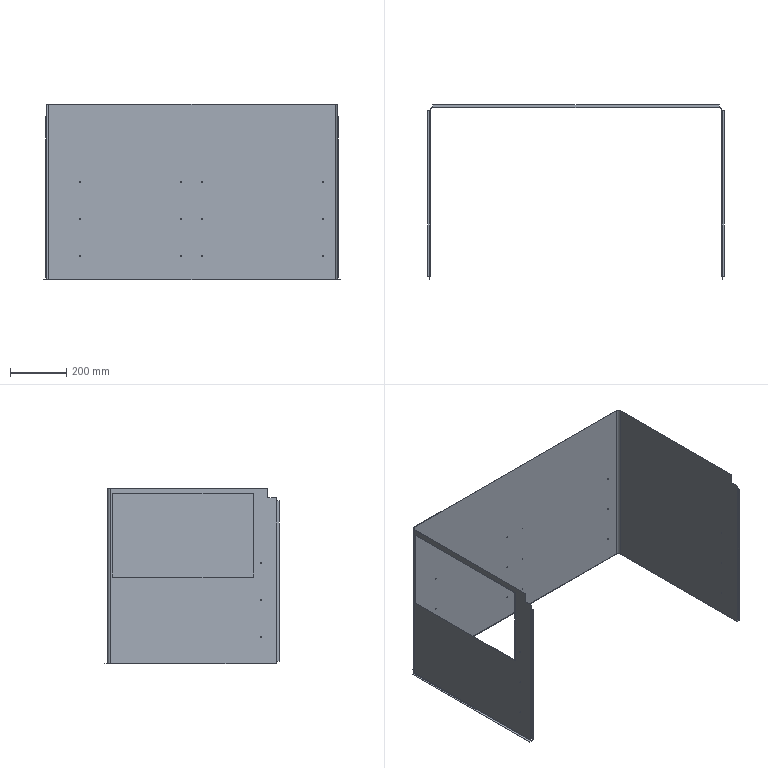Part | SolidWorks | features ICE 6, EdgeFlange 3, FlatPattern 1, SMBaseFlange 1, SheetMetal 1, UnFold 1 | 1 solid | 142 faces | box 1056 x 619.4 x 625.6 mm | volume 765945 mm3 | plane 88 | cylinder 54 | commonest cylinder face diameters 3.25 x36 0.2 x4 1.4 x4 1.473 x3 2.673 x3 18.8 x2